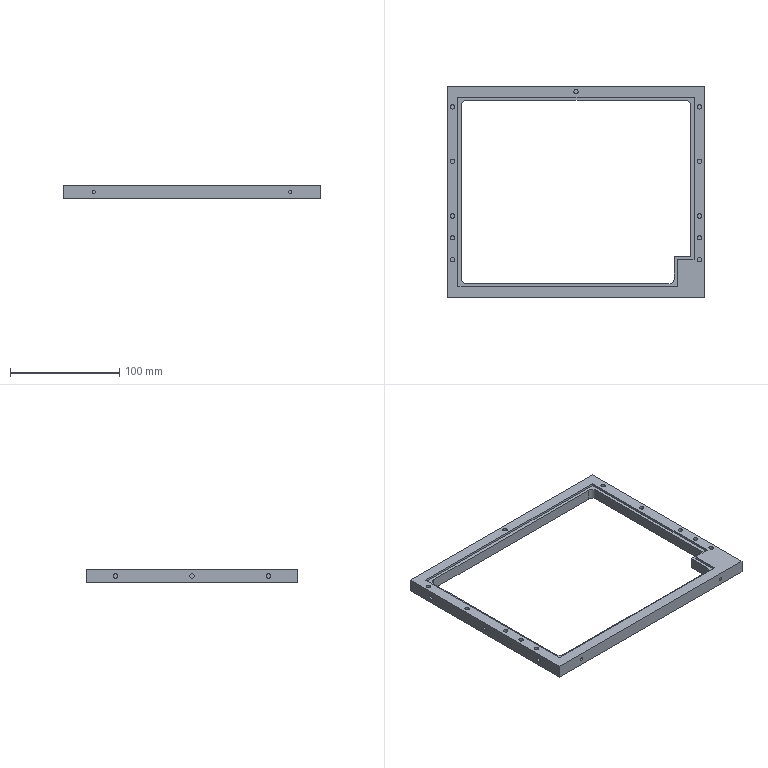Part | SolidWorks | features ICE 6, MirrorPattern 3, Extrusion 1, Fillet 1 | 1 solid | 86 faces | box 236.3 x 194 x 12 mm | volume 125428 mm3 | cylinder 46 | plane 40 | commonest cylinder face diameters 4 x34 3 x8 10 x4